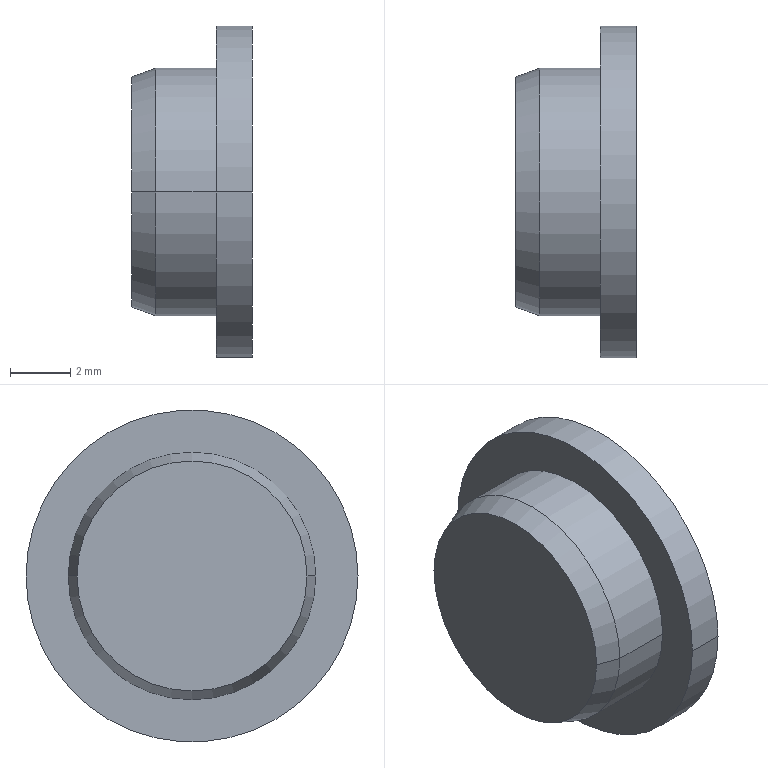Part | NX | features BREP 1 | 1 solid | 9 faces | box 4 x 11 x 11 mm | volume 258.979 mm3 | cylinder 4 | plane 3 | cone 2 | commonest cylinder face diameters 8.2 x2 11 x2
STEP:
#1=CARTESIAN_POINT('',(172.467,55.413,13.444));
#2=VERTEX_POINT('',#1);
#3=CARTESIAN_POINT('',(172.467,66.413,13.444));
#4=VERTEX_POINT('',#3);
#5=CARTESIAN_POINT('',(172.467,60.913,13.444));
#6=DIRECTION('',(-1.,0.,0.));
#7=DIRECTION('',(0.,-1.,0.));
#8=AXIS2_PLACEMENT_3D('',#5,#6,#7);
#9=CIRCLE('',#8,5.5);
#10=EDGE_CURVE('',#2,#4,#9,.T.);
#11=ORIENTED_EDGE('',*,*,#10,.T.);
#12=CARTESIAN_POINT('',(171.267,66.413,13.444));
#13=VERTEX_POINT('',#12);
#14=CARTESIAN_POINT('',(168.467,66.413,13.444));
#15=DIRECTION('',(-1.,0.,0.));
#16=VECTOR('',#15,1000.);
#17=LINE('',#14,#16);
#18=EDGE_CURVE('',#4,#13,#17,.T.);
#19=ORIENTED_EDGE('',*,*,#18,.T.);
#20=CARTESIAN_POINT('',(171.267,55.413,13.444));
#21=VERTEX_POINT('',#20);
#22=CARTESIAN_POINT('',(171.267,60.913,13.444));
#23=DIRECTION('',(1.,0.,0.));
#24=DIRECTION('',(0.,-1.,0.));
#25=AXIS2_PLACEMENT_3D('',#22,#23,#24);
#26=CIRCLE('',#25,5.5);
#27=EDGE_CURVE('',#13,#21,#26,.T.);
#28=ORIENTED_EDGE('',*,*,#27,.T.);
#29=CARTESIAN_POINT('',(168.467,55.413,13.444));
#30=DIRECTION('',(-1.,0.,0.));
#31=VECTOR('',#30,1000.);
#32=LINE('',#29,#31);
#33=EDGE_CURVE('',#2,#21,#32,.T.);
#34=ORIENTED_EDGE('',*,*,#33,.F.);
#35=EDGE_LOOP('',(#11,#19,#28,#34));
#36=FACE_BOUND('',#35,.T.);
#37=CARTESIAN_POINT('',(168.467,60.913,13.444));
#38=DIRECTION('',(-1.,0.,0.));
#39=DIRECTION('',(0.,-1.,0.));
#40=AXIS2_PLACEMENT_3D('',#37,#38,#39);
#41=CYLINDRICAL_SURFACE('',#40,5.5);
#42=ADVANCED_FACE('',(#36),#41,.T.);
#43=CARTESIAN_POINT('',(171.267,56.813,13.444));
#44=VERTEX_POINT('',#43);
#45=CARTESIAN_POINT('',(171.267,65.013,13.444));
#46=VERTEX_POINT('',#45);
#47=CARTESIAN_POINT('',(171.267,60.913,13.444));
#48=DIRECTION('',(-1.,0.,0.));
#49=DIRECTION('',(0.,-1.,0.));
#50=AXIS2_PLACEMENT_3D('',#47,#48,#49);
#51=CIRCLE('',#50,4.1);
#52=EDGE_CURVE('',#44,#46,#51,.T.);
#53=ORIENTED_EDGE('',*,*,#52,.T.);
#54=CARTESIAN_POINT('',(169.267,65.013,13.444));
#55=VERTEX_POINT('',#54);
#56=CARTESIAN_POINT('',(168.467,65.013,13.444));
#57=DIRECTION('',(-1.,0.,0.));
#58=VECTOR('',#57,1000.);
#59=LINE('',#56,#58);
#60=EDGE_CURVE('',#46,#55,#59,.T.);
#61=ORIENTED_EDGE('',*,*,#60,.T.);
#62=CARTESIAN_POINT('',(169.267,56.813,13.444));
#63=VERTEX_POINT('',#62);
#64=CARTESIAN_POINT('',(169.267,60.913,13.444));
#65=DIRECTION('',(1.,0.,0.));
#66=DIRECTION('',(0.,-1.,0.));
#67=AXIS2_PLACEMENT_3D('',#64,#65,#66);
#68=CIRCLE('',#67,4.1);
#69=EDGE_CURVE('',#55,#63,#68,.T.);
#70=ORIENTED_EDGE('',*,*,#69,.T.);
#71=CARTESIAN_POINT('',(168.467,56.813,13.444));
#72=DIRECTION('',(-1.,0.,0.));
#73=VECTOR('',#72,1000.);
#74=LINE('',#71,#73);
#75=EDGE_CURVE('',#44,#63,#74,.T.);
#76=ORIENTED_EDGE('',*,*,#75,.F.);
#77=EDGE_LOOP('',(#53,#61,#70,#76));
#78=FACE_BOUND('',#77,.T.);
#79=CARTESIAN_POINT('',(168.467,60.913,13.444));
#80=DIRECTION('',(-1.,0.,0.));
#81=DIRECTION('',(0.,-1.,0.));
#82=AXIS2_PLACEMENT_3D('',#79,#80,#81);
#83=CYLINDRICAL_SURFACE('',#82,4.1);
#84=ADVANCED_FACE('',(#78),#83,.T.);
#85=CARTESIAN_POINT('',(168.467,64.722,13.444));
#86=VERTEX_POINT('',#85);
#87=CARTESIAN_POINT('',(168.467,57.104,13.444));
#88=VERTEX_POINT('',#87);
#89=CARTESIAN_POINT('',(168.467,60.913,13.444));
#90=DIRECTION('',(1.,0.,0.));
#91=DIRECTION('',(0.,1.,0.));
#92=AXIS2_PLACEMENT_3D('',#89,#90,#91);
#93=CIRCLE('',#92,3.809);
#94=EDGE_CURVE('',#86,#88,#93,.T.);
#95=ORIENTED_EDGE('',*,*,#94,.T.);
#96=CARTESIAN_POINT('',(169.267,56.813,13.444));
#97=DIRECTION('',(0.9397,-0.342,0.));
#98=VECTOR('',#97,1000.);
#99=LINE('',#96,#98);
#100=EDGE_CURVE('',#63,#88,#99,.F.);
#101=ORIENTED_EDGE('',*,*,#100,.F.);
#102=ORIENTED_EDGE('',*,*,#69,.F.);
#103=CARTESIAN_POINT('',(169.267,65.013,13.444));
#104=DIRECTION('',(0.9397,0.342,0.));
#105=VECTOR('',#104,1000.);
#106=LINE('',#103,#105);
#107=EDGE_CURVE('',#55,#86,#106,.F.);
#108=ORIENTED_EDGE('',*,*,#107,.T.);
#109=EDGE_LOOP('',(#95,#101,#102,#108));
#110=FACE_BOUND('',#109,.T.);
#111=CARTESIAN_POINT('',(169.267,60.913,13.444));
#112=DIRECTION('',(1.,0.,0.));
#113=DIRECTION('',(0.,1.,0.));
#114=AXIS2_PLACEMENT_3D('',#111,#112,#113);
#115=CONICAL_SURFACE('',#114,4.1,0.3491);
#116=ADVANCED_FACE('',(#110),#115,.T.);
#117=ORIENTED_EDGE('',*,*,#10,.F.);
#118=CARTESIAN_POINT('',(172.467,60.913,13.444));
#119=DIRECTION('',(-1.,0.,0.));
#120=DIRECTION('',(0.,-1.,0.));
#121=AXIS2_PLACEMENT_3D('',#118,#119,#120);
#122=CIRCLE('',#121,5.5);
#123=EDGE_CURVE('',#4,#2,#122,.T.);
#124=ORIENTED_EDGE('',*,*,#123,.F.);
#125=EDGE_LOOP('',(#117,#124));
#126=FACE_BOUND('',#125,.T.);
#127=CARTESIAN_POINT('',(172.467,60.913,13.444));
#128=DIRECTION('',(-1.,0.,0.));
#129=DIRECTION('',(0.,0.,1.));
#130=AXIS2_PLACEMENT_3D('',#127,#128,#129);
#131=PLANE('',#130);
#132=ADVANCED_FACE('',(#126),#131,.F.);
#133=ORIENTED_EDGE('',*,*,#18,.F.);
#134=ORIENTED_EDGE('',*,*,#123,.T.);
#135=ORIENTED_EDGE('',*,*,#33,.T.);
#136=CARTESIAN_POINT('',(171.267,60.913,13.444));
#137=DIRECTION('',(1.,0.,0.));
#138=DIRECTION('',(0.,-1.,0.));
#139=AXIS2_PLACEMENT_3D('',#136,#137,#138);
#140=CIRCLE('',#139,5.5);
#141=EDGE_CURVE('',#21,#13,#140,.T.);
#142=ORIENTED_EDGE('',*,*,#141,.T.);
#143=EDGE_LOOP('',(#133,#134,#135,#142));
#144=FACE_BOUND('',#143,.T.);
#145=CARTESIAN_POINT('',(168.467,60.913,13.444));
#146=DIRECTION('',(-1.,0.,0.));
#147=DIRECTION('',(0.,-1.,0.));
#148=AXIS2_PLACEMENT_3D('',#145,#146,#147);
#149=CYLINDRICAL_SURFACE('',#148,5.5);
#150=ADVANCED_FACE('',(#144),#149,.T.);
#151=ORIENTED_EDGE('',*,*,#141,.F.);
#152=ORIENTED_EDGE('',*,*,#27,.F.);
#153=EDGE_LOOP('',(#151,#152));
#154=FACE_BOUND('',#153,.T.);
#155=ORIENTED_EDGE('',*,*,#52,.F.);
#156=CARTESIAN_POINT('',(171.267,60.913,13.444));
#157=DIRECTION('',(-1.,0.,0.));
#158=DIRECTION('',(0.,-1.,0.));
#159=AXIS2_PLACEMENT_3D('',#156,#157,#158);
#160=CIRCLE('',#159,4.1);
#161=EDGE_CURVE('',#46,#44,#160,.T.);
#162=ORIENTED_EDGE('',*,*,#161,.F.);
#163=EDGE_LOOP('',(#155,#162));
#164=FACE_BOUND('',#163,.T.);
#165=CARTESIAN_POINT('',(171.267,66.413,13.444));
#166=DIRECTION('',(1.,0.,0.));
#167=DIRECTION('',(0.,-1.,0.));
#168=AXIS2_PLACEMENT_3D('',#165,#166,#167);
#169=PLANE('',#168);
#170=ADVANCED_FACE('',(#154,#164),#169,.F.);
#171=ORIENTED_EDGE('',*,*,#60,.F.);
#172=ORIENTED_EDGE('',*,*,#161,.T.);
#173=ORIENTED_EDGE('',*,*,#75,.T.);
#174=CARTESIAN_POINT('',(169.267,60.913,13.444));
#175=DIRECTION('',(1.,0.,0.));
#176=DIRECTION('',(0.,-1.,0.));
#177=AXIS2_PLACEMENT_3D('',#174,#175,#176);
#178=CIRCLE('',#177,4.1);
#179=EDGE_CURVE('',#63,#55,#178,.T.);
#180=ORIENTED_EDGE('',*,*,#179,.T.);
#181=EDGE_LOOP('',(#171,#172,#173,#180));
#182=FACE_BOUND('',#181,.T.);
#183=CARTESIAN_POINT('',(168.467,60.913,13.444));
#184=DIRECTION('',(-1.,0.,0.));
#185=DIRECTION('',(0.,-1.,0.));
#186=AXIS2_PLACEMENT_3D('',#183,#184,#185);
#187=CYLINDRICAL_SURFACE('',#186,4.1);
#188=ADVANCED_FACE('',(#182),#187,.T.);
#189=ORIENTED_EDGE('',*,*,#100,.T.);
#190=CARTESIAN_POINT('',(168.467,60.913,13.444));
#191=DIRECTION('',(1.,0.,0.));
#192=DIRECTION('',(0.,1.,0.));
#193=AXIS2_PLACEMENT_3D('',#190,#191,#192);
#194=CIRCLE('',#193,3.809);
#195=EDGE_CURVE('',#88,#86,#194,.T.);
#196=ORIENTED_EDGE('',*,*,#195,.T.);
#197=ORIENTED_EDGE('',*,*,#107,.F.);
#198=ORIENTED_EDGE('',*,*,#179,.F.);
#199=EDGE_LOOP('',(#189,#196,#197,#198));
#200=FACE_BOUND('',#199,.T.);
#201=CARTESIAN_POINT('',(169.267,60.913,13.444));
#202=DIRECTION('',(1.,0.,0.));
#203=DIRECTION('',(0.,1.,0.));
#204=AXIS2_PLACEMENT_3D('',#201,#202,#203);
#205=CONICAL_SURFACE('',#204,4.1,0.3491);
#206=ADVANCED_FACE('',(#200),#205,.T.);
#207=ORIENTED_EDGE('',*,*,#94,.F.);
#208=ORIENTED_EDGE('',*,*,#195,.F.);
#209=EDGE_LOOP('',(#207,#208));
#210=FACE_BOUND('',#209,.T.);
#211=CARTESIAN_POINT('',(168.467,65.013,13.444));
#212=DIRECTION('',(1.,0.,0.));
#213=DIRECTION('',(0.,-1.,0.));
#214=AXIS2_PLACEMENT_3D('',#211,#212,#213);
#215=PLANE('',#214);
#216=ADVANCED_FACE('',(#210),#215,.F.);
#217=CLOSED_SHELL('',(#42,#84,#116,#132,#150,#170,#188,#206,#216));
#218=MANIFOLD_SOLID_BREP('',#217);
#219=(LENGTH_UNIT()NAMED_UNIT(*)SI_UNIT(.MILLI.,.METRE.));
#220=UNCERTAINTY_MEASURE_WITH_UNIT(LENGTH_MEASURE(0.00001),#219,'','');
#221=(NAMED_UNIT(*)PLANE_ANGLE_UNIT()SI_UNIT($,.RADIAN.));
#222=(NAMED_UNIT(*)SI_UNIT($,.STERADIAN.)SOLID_ANGLE_UNIT());
#223=(GEOMETRIC_REPRESENTATION_CONTEXT(3)GLOBAL_UNCERTAINTY_ASSIGNED_CONTEXT((#220))GLOBAL_UNIT_ASSIGNED_CONTEXT((#219,#221,#222))REPRESENTATION_CONTEXT('',''));
#224=ADVANCED_BREP_SHAPE_REPRESENTATION('',(#218),#223);